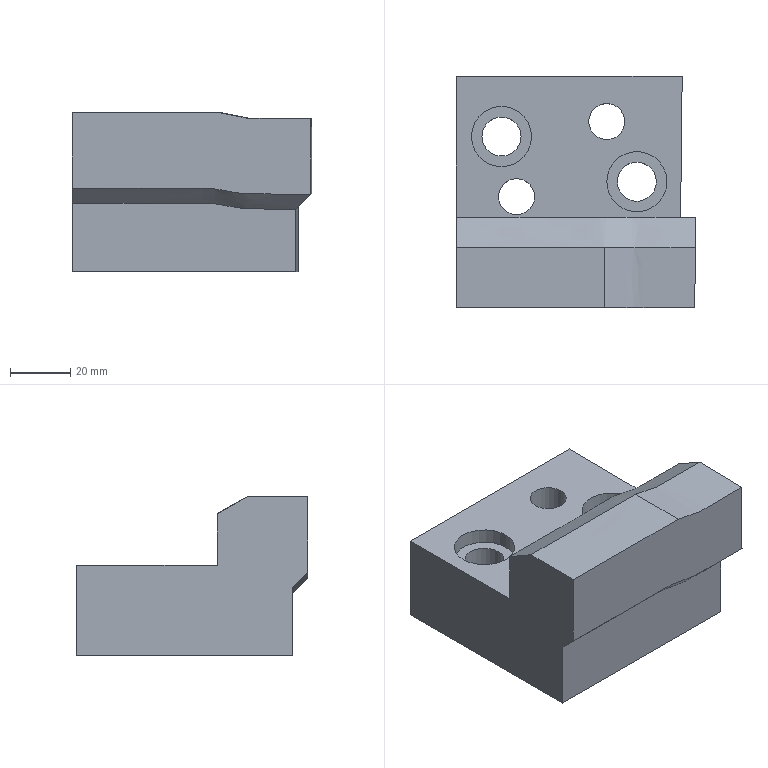Part | NX | features solid 2 | 1 solid | 23 faces | box 79.545 x 76.857 x 52.876 mm | volume 197901 mm3 | plane 9 | spline 8 | cylinder 6 | commonest cylinder face diameters 12 x2 13 x2 20 x2